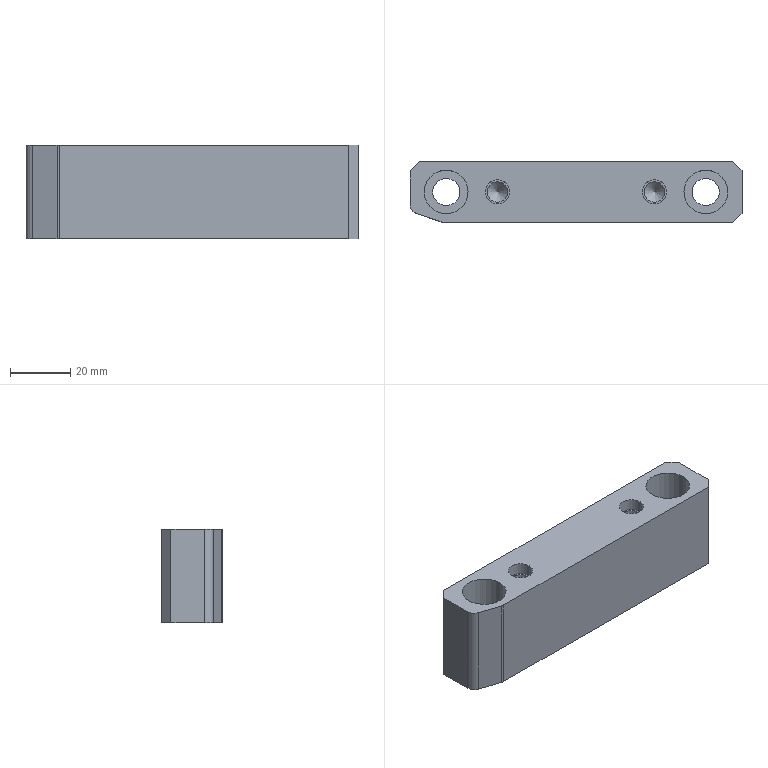Part | NX | features DIE-51 2 | 1 solid | 26 faces | box 110 x 20 x 31 mm | volume 58925 mm3 | plane 14 | cylinder 10 | cone 2 | commonest cylinder face diameters 6 x2 6.806 x2 8 x2 9 x2 14.5 x2
STEP:
#1=CARTESIAN_POINT('',(3332.094,-787.623,884.716));
#2=VERTEX_POINT('',#1);
#3=CARTESIAN_POINT('',(3336.094,-787.623,884.716));
#4=DIRECTION('',(0.,0.,1.));
#5=DIRECTION('',(-1.,0.,0.));
#6=AXIS2_PLACEMENT_3D('',#3,#4,#5);
#7=CIRCLE('',#6,4.);
#8=EDGE_CURVE('',#2,#2,#7,.T.);
#9=ORIENTED_EDGE('',*,*,#8,.F.);
#10=EDGE_LOOP('',(#9));
#11=FACE_BOUND('',#10,.T.);
#12=CARTESIAN_POINT('',(3392.094,-787.623,884.716));
#13=VERTEX_POINT('',#12);
#14=CARTESIAN_POINT('',(3388.094,-787.623,884.716));
#15=DIRECTION('',(0.,0.,-1.));
#16=DIRECTION('',(1.,0.,0.));
#17=AXIS2_PLACEMENT_3D('',#14,#15,#16);
#18=CIRCLE('',#17,4.);
#19=EDGE_CURVE('',#13,#13,#18,.T.);
#20=ORIENTED_EDGE('',*,*,#19,.T.);
#21=EDGE_LOOP('',(#20));
#22=FACE_BOUND('',#21,.T.);
#23=CARTESIAN_POINT('',(3412.344,-787.623,884.716));
#24=VERTEX_POINT('',#23);
#25=CARTESIAN_POINT('',(3405.094,-787.623,884.716));
#26=DIRECTION('',(0.,0.,1.));
#27=DIRECTION('',(1.,0.,0.));
#28=AXIS2_PLACEMENT_3D('',#25,#26,#27);
#29=CIRCLE('',#28,7.25);
#30=EDGE_CURVE('',#24,#24,#29,.T.);
#31=ORIENTED_EDGE('',*,*,#30,.F.);
#32=EDGE_LOOP('',(#31));
#33=FACE_BOUND('',#32,.T.);
#34=CARTESIAN_POINT('',(3326.344,-787.623,884.716));
#35=VERTEX_POINT('',#34);
#36=CARTESIAN_POINT('',(3319.094,-787.623,884.716));
#37=DIRECTION('',(0.,0.,1.));
#38=DIRECTION('',(1.,0.,0.));
#39=AXIS2_PLACEMENT_3D('',#36,#37,#38);
#40=CIRCLE('',#39,7.25);
#41=EDGE_CURVE('',#35,#35,#40,.T.);
#42=ORIENTED_EDGE('',*,*,#41,.F.);
#43=EDGE_LOOP('',(#42));
#44=FACE_BOUND('',#43,.T.);
#45=CARTESIAN_POINT('',(3317.375,-797.469,884.716));
#46=VERTEX_POINT('',#45);
#47=CARTESIAN_POINT('',(3309.145,-794.725,884.716));
#48=VERTEX_POINT('',#47);
#49=CARTESIAN_POINT('',(3313.568,-796.2,884.716));
#50=DIRECTION('',(0.9487,-0.3162,0.));
#51=VECTOR('',#50,1000.);
#52=LINE('',#49,#51);
#53=EDGE_CURVE('',#46,#48,#52,.F.);
#54=ORIENTED_EDGE('',*,*,#53,.F.);
#55=CARTESIAN_POINT('',(3318.324,-797.623,884.716));
#56=VERTEX_POINT('',#55);
#57=CARTESIAN_POINT('',(3318.324,-794.623,884.716));
#58=DIRECTION('',(0.,0.,-1.));
#59=DIRECTION('',(1.,0.,0.));
#60=AXIS2_PLACEMENT_3D('',#57,#58,#59);
#61=CIRCLE('',#60,3.);
#62=EDGE_CURVE('',#56,#46,#61,.T.);
#63=ORIENTED_EDGE('',*,*,#62,.F.);
#64=CARTESIAN_POINT('',(3414.094,-797.623,884.716));
#65=VERTEX_POINT('',#64);
#66=CARTESIAN_POINT('',(3322.094,-797.623,884.716));
#67=DIRECTION('',(1.,0.,0.));
#68=VECTOR('',#67,1000.);
#69=LINE('',#66,#68);
#70=EDGE_CURVE('',#56,#65,#69,.T.);
#71=ORIENTED_EDGE('',*,*,#70,.T.);
#72=CARTESIAN_POINT('',(3417.094,-794.623,884.716));
#73=VERTEX_POINT('',#72);
#74=CARTESIAN_POINT('',(3373.094,-838.623,884.716));
#75=DIRECTION('',(0.7071,0.7071,0.));
#76=VECTOR('',#75,1000.);
#77=LINE('',#74,#76);
#78=EDGE_CURVE('',#73,#65,#77,.F.);
#79=ORIENTED_EDGE('',*,*,#78,.F.);
#80=CARTESIAN_POINT('',(3417.094,-780.623,884.716));
#81=VERTEX_POINT('',#80);
#82=CARTESIAN_POINT('',(3417.094,-787.623,884.716));
#83=DIRECTION('',(0.,1.,0.));
#84=VECTOR('',#83,1000.);
#85=LINE('',#82,#84);
#86=EDGE_CURVE('',#73,#81,#85,.T.);
#87=ORIENTED_EDGE('',*,*,#86,.T.);
#88=CARTESIAN_POINT('',(3414.094,-777.623,884.716));
#89=VERTEX_POINT('',#88);
#90=CARTESIAN_POINT('',(3373.094,-736.623,884.716));
#91=DIRECTION('',(-0.7071,0.7071,0.));
#92=VECTOR('',#91,1000.);
#93=LINE('',#90,#92);
#94=EDGE_CURVE('',#89,#81,#93,.F.);
#95=ORIENTED_EDGE('',*,*,#94,.F.);
#96=CARTESIAN_POINT('',(3310.094,-777.623,884.716));
#97=VERTEX_POINT('',#96);
#98=CARTESIAN_POINT('',(3322.094,-777.623,884.716));
#99=DIRECTION('',(-1.,0.,0.));
#100=VECTOR('',#99,1000.);
#101=LINE('',#98,#100);
#102=EDGE_CURVE('',#89,#97,#101,.T.);
#103=ORIENTED_EDGE('',*,*,#102,.T.);
#104=CARTESIAN_POINT('',(3307.094,-780.623,884.716));
#105=VERTEX_POINT('',#104);
#106=CARTESIAN_POINT('',(3311.094,-776.623,884.716));
#107=DIRECTION('',(-0.7071,-0.7071,0.));
#108=VECTOR('',#107,1000.);
#109=LINE('',#106,#108);
#110=EDGE_CURVE('',#105,#97,#109,.F.);
#111=ORIENTED_EDGE('',*,*,#110,.F.);
#112=CARTESIAN_POINT('',(3307.094,-791.879,884.716));
#113=VERTEX_POINT('',#112);
#114=CARTESIAN_POINT('',(3307.094,-787.623,884.716));
#115=DIRECTION('',(0.,-1.,0.));
#116=VECTOR('',#115,1000.);
#117=LINE('',#114,#116);
#118=EDGE_CURVE('',#105,#113,#117,.T.);
#119=ORIENTED_EDGE('',*,*,#118,.T.);
#120=CARTESIAN_POINT('',(3310.094,-791.879,884.716));
#121=DIRECTION('',(0.,0.,-1.));
#122=DIRECTION('',(1.,0.,0.));
#123=AXIS2_PLACEMENT_3D('',#120,#121,#122);
#124=CIRCLE('',#123,3.);
#125=EDGE_CURVE('',#48,#113,#124,.T.);
#126=ORIENTED_EDGE('',*,*,#125,.F.);
#127=EDGE_LOOP('',(#54,#63,#71,#79,#87,#95,#103,#111,#119,#126));
#128=FACE_BOUND('',#127,.T.);
#129=CARTESIAN_POINT('',(3322.094,-787.623,884.716));
#130=DIRECTION('',(0.,0.,1.));
#131=DIRECTION('',(1.,0.,0.));
#132=AXIS2_PLACEMENT_3D('',#129,#130,#131);
#133=PLANE('',#132);
#134=ADVANCED_FACE('',(#11,#22,#33,#44,#128),#133,.T.);
#135=CARTESIAN_POINT('',(3310.094,-777.623,853.716));
#136=VERTEX_POINT('',#135);
#137=CARTESIAN_POINT('',(3414.094,-777.623,853.716));
#138=VERTEX_POINT('',#137);
#139=CARTESIAN_POINT('',(3322.094,-777.623,853.716));
#140=DIRECTION('',(1.,0.,0.));
#141=VECTOR('',#140,1000.);
#142=LINE('',#139,#141);
#143=EDGE_CURVE('',#136,#138,#142,.T.);
#144=ORIENTED_EDGE('',*,*,#143,.F.);
#145=CARTESIAN_POINT('',(3310.094,-777.623,841.716));
#146=DIRECTION('',(0.,0.,-1.));
#147=VECTOR('',#146,1000.);
#148=LINE('',#145,#147);
#149=EDGE_CURVE('',#97,#136,#148,.T.);
#150=ORIENTED_EDGE('',*,*,#149,.F.);
#151=ORIENTED_EDGE('',*,*,#102,.F.);
#152=CARTESIAN_POINT('',(3414.094,-777.623,841.716));
#153=DIRECTION('',(0.,0.,-1.));
#154=VECTOR('',#153,1000.);
#155=LINE('',#152,#154);
#156=EDGE_CURVE('',#138,#89,#155,.F.);
#157=ORIENTED_EDGE('',*,*,#156,.F.);
#158=EDGE_LOOP('',(#144,#150,#151,#157));
#159=FACE_BOUND('',#158,.T.);
#160=CARTESIAN_POINT('',(3322.094,-777.623,841.716));
#161=DIRECTION('',(0.,1.,0.));
#162=DIRECTION('',(0.,0.,-1.));
#163=AXIS2_PLACEMENT_3D('',#160,#161,#162);
#164=PLANE('',#163);
#165=ADVANCED_FACE('',(#159),#164,.T.);
#166=ORIENTED_EDGE('',*,*,#118,.F.);
#167=CARTESIAN_POINT('',(3307.094,-780.623,853.716));
#168=VERTEX_POINT('',#167);
#169=CARTESIAN_POINT('',(3307.094,-780.623,841.716));
#170=DIRECTION('',(0.,0.,1.));
#171=VECTOR('',#170,1000.);
#172=LINE('',#169,#171);
#173=EDGE_CURVE('',#168,#105,#172,.T.);
#174=ORIENTED_EDGE('',*,*,#173,.F.);
#175=CARTESIAN_POINT('',(3307.094,-791.879,853.716));
#176=VERTEX_POINT('',#175);
#177=CARTESIAN_POINT('',(3307.094,-787.623,853.716));
#178=DIRECTION('',(0.,1.,0.));
#179=VECTOR('',#178,1000.);
#180=LINE('',#177,#179);
#181=EDGE_CURVE('',#176,#168,#180,.T.);
#182=ORIENTED_EDGE('',*,*,#181,.F.);
#183=CARTESIAN_POINT('',(3307.094,-791.879,841.716));
#184=DIRECTION('',(0.,0.,1.));
#185=VECTOR('',#184,1000.);
#186=LINE('',#183,#185);
#187=EDGE_CURVE('',#113,#176,#186,.F.);
#188=ORIENTED_EDGE('',*,*,#187,.F.);
#189=EDGE_LOOP('',(#166,#174,#182,#188));
#190=FACE_BOUND('',#189,.T.);
#191=CARTESIAN_POINT('',(3307.094,-787.623,841.716));
#192=DIRECTION('',(-1.,0.,0.));
#193=DIRECTION('',(0.,0.,1.));
#194=AXIS2_PLACEMENT_3D('',#191,#192,#193);
#195=PLANE('',#194);
#196=ADVANCED_FACE('',(#190),#195,.T.);
#197=CARTESIAN_POINT('',(3414.094,-797.623,853.716));
#198=VERTEX_POINT('',#197);
#199=CARTESIAN_POINT('',(3318.324,-797.623,853.716));
#200=VERTEX_POINT('',#199);
#201=CARTESIAN_POINT('',(3322.094,-797.623,853.716));
#202=DIRECTION('',(-1.,0.,0.));
#203=VECTOR('',#202,1000.);
#204=LINE('',#201,#203);
#205=EDGE_CURVE('',#198,#200,#204,.T.);
#206=ORIENTED_EDGE('',*,*,#205,.F.);
#207=CARTESIAN_POINT('',(3414.094,-797.623,841.716));
#208=DIRECTION('',(0.,0.,1.));
#209=VECTOR('',#208,1000.);
#210=LINE('',#207,#209);
#211=EDGE_CURVE('',#65,#198,#210,.F.);
#212=ORIENTED_EDGE('',*,*,#211,.F.);
#213=ORIENTED_EDGE('',*,*,#70,.F.);
#214=CARTESIAN_POINT('',(3318.324,-797.623,841.716));
#215=DIRECTION('',(0.,0.,-1.));
#216=VECTOR('',#215,1000.);
#217=LINE('',#214,#216);
#218=EDGE_CURVE('',#200,#56,#217,.F.);
#219=ORIENTED_EDGE('',*,*,#218,.F.);
#220=EDGE_LOOP('',(#206,#212,#213,#219));
#221=FACE_BOUND('',#220,.T.);
#222=CARTESIAN_POINT('',(3322.094,-797.623,841.716));
#223=DIRECTION('',(0.,-1.,0.));
#224=DIRECTION('',(0.,0.,1.));
#225=AXIS2_PLACEMENT_3D('',#222,#223,#224);
#226=PLANE('',#225);
#227=ADVANCED_FACE('',(#221),#226,.T.);
#228=CARTESIAN_POINT('',(3400.594,-787.623,853.716));
#229=VERTEX_POINT('',#228);
#230=CARTESIAN_POINT('',(3405.094,-787.623,853.716));
#231=DIRECTION('',(0.,0.,-1.));
#232=DIRECTION('',(-1.,0.,0.));
#233=AXIS2_PLACEMENT_3D('',#230,#231,#232);
#234=CIRCLE('',#233,4.5);
#235=EDGE_CURVE('',#229,#229,#234,.T.);
#236=ORIENTED_EDGE('',*,*,#235,.F.);
#237=EDGE_LOOP('',(#236));
#238=FACE_BOUND('',#237,.T.);
#239=CARTESIAN_POINT('',(3314.594,-787.623,853.716));
#240=VERTEX_POINT('',#239);
#241=CARTESIAN_POINT('',(3319.094,-787.623,853.716));
#242=DIRECTION('',(0.,0.,-1.));
#243=DIRECTION('',(-1.,0.,0.));
#244=AXIS2_PLACEMENT_3D('',#241,#242,#243);
#245=CIRCLE('',#244,4.5);
#246=EDGE_CURVE('',#240,#240,#245,.T.);
#247=ORIENTED_EDGE('',*,*,#246,.F.);
#248=EDGE_LOOP('',(#247));
#249=FACE_BOUND('',#248,.T.);
#250=ORIENTED_EDGE('',*,*,#181,.T.);
#251=CARTESIAN_POINT('',(3307.094,-780.623,853.716));
#252=DIRECTION('',(0.7071,0.7071,0.));
#253=VECTOR('',#252,1000.);
#254=LINE('',#251,#253);
#255=EDGE_CURVE('',#136,#168,#254,.F.);
#256=ORIENTED_EDGE('',*,*,#255,.F.);
#257=ORIENTED_EDGE('',*,*,#143,.T.);
#258=CARTESIAN_POINT('',(3417.094,-780.623,853.716));
#259=VERTEX_POINT('',#258);
#260=CARTESIAN_POINT('',(3414.094,-777.623,853.716));
#261=DIRECTION('',(0.7071,-0.7071,0.));
#262=VECTOR('',#261,1000.);
#263=LINE('',#260,#262);
#264=EDGE_CURVE('',#259,#138,#263,.F.);
#265=ORIENTED_EDGE('',*,*,#264,.F.);
#266=CARTESIAN_POINT('',(3417.094,-794.623,853.716));
#267=VERTEX_POINT('',#266);
#268=CARTESIAN_POINT('',(3417.094,-787.623,853.716));
#269=DIRECTION('',(0.,-1.,0.));
#270=VECTOR('',#269,1000.);
#271=LINE('',#268,#270);
#272=EDGE_CURVE('',#259,#267,#271,.T.);
#273=ORIENTED_EDGE('',*,*,#272,.T.);
#274=CARTESIAN_POINT('',(3417.094,-794.623,853.716));
#275=DIRECTION('',(-0.7071,-0.7071,0.));
#276=VECTOR('',#275,1000.);
#277=LINE('',#274,#276);
#278=EDGE_CURVE('',#198,#267,#277,.F.);
#279=ORIENTED_EDGE('',*,*,#278,.F.);
#280=ORIENTED_EDGE('',*,*,#205,.T.);
#281=CARTESIAN_POINT('',(3317.375,-797.469,853.716));
#282=VERTEX_POINT('',#281);
#283=CARTESIAN_POINT('',(3318.324,-794.623,853.716));
#284=DIRECTION('',(0.,0.,-1.));
#285=DIRECTION('',(-1.,0.,0.));
#286=AXIS2_PLACEMENT_3D('',#283,#284,#285);
#287=CIRCLE('',#286,3.);
#288=EDGE_CURVE('',#282,#200,#287,.F.);
#289=ORIENTED_EDGE('',*,*,#288,.F.);
#290=CARTESIAN_POINT('',(3309.145,-794.725,853.716));
#291=VERTEX_POINT('',#290);
#292=CARTESIAN_POINT('',(3313.568,-796.2,853.716));
#293=DIRECTION('',(-0.9487,0.3162,0.));
#294=VECTOR('',#293,1000.);
#295=LINE('',#292,#294);
#296=EDGE_CURVE('',#291,#282,#295,.F.);
#297=ORIENTED_EDGE('',*,*,#296,.F.);
#298=CARTESIAN_POINT('',(3310.094,-791.879,853.716));
#299=DIRECTION('',(0.,0.,-1.));
#300=DIRECTION('',(-1.,0.,0.));
#301=AXIS2_PLACEMENT_3D('',#298,#299,#300);
#302=CIRCLE('',#301,3.);
#303=EDGE_CURVE('',#176,#291,#302,.F.);
#304=ORIENTED_EDGE('',*,*,#303,.F.);
#305=EDGE_LOOP('',(#250,#256,#257,#265,#273,#279,#280,#289,#297,#304));
#306=FACE_BOUND('',#305,.T.);
#307=CARTESIAN_POINT('',(3322.094,-787.623,853.716));
#308=DIRECTION('',(0.,0.,-1.));
#309=DIRECTION('',(-1.,0.,0.));
#310=AXIS2_PLACEMENT_3D('',#307,#308,#309);
#311=PLANE('',#310);
#312=ADVANCED_FACE('',(#238,#249,#306),#311,.T.);
#313=ORIENTED_EDGE('',*,*,#272,.F.);
#314=CARTESIAN_POINT('',(3417.094,-780.623,841.716));
#315=DIRECTION('',(0.,0.,1.));
#316=VECTOR('',#315,1000.);
#317=LINE('',#314,#316);
#318=EDGE_CURVE('',#81,#259,#317,.F.);
#319=ORIENTED_EDGE('',*,*,#318,.F.);
#320=ORIENTED_EDGE('',*,*,#86,.F.);
#321=CARTESIAN_POINT('',(3417.094,-794.623,841.716));
#322=DIRECTION('',(0.,0.,-1.));
#323=VECTOR('',#322,1000.);
#324=LINE('',#321,#323);
#325=EDGE_CURVE('',#267,#73,#324,.F.);
#326=ORIENTED_EDGE('',*,*,#325,.F.);
#327=EDGE_LOOP('',(#313,#319,#320,#326));
#328=FACE_BOUND('',#327,.T.);
#329=CARTESIAN_POINT('',(3417.094,-787.623,841.716));
#330=DIRECTION('',(1.,0.,0.));
#331=DIRECTION('',(0.,0.,-1.));
#332=AXIS2_PLACEMENT_3D('',#329,#330,#331);
#333=PLANE('',#332);
#334=ADVANCED_FACE('',(#328),#333,.T.);
#335=ORIENTED_EDGE('',*,*,#264,.T.);
#336=ORIENTED_EDGE('',*,*,#156,.T.);
#337=ORIENTED_EDGE('',*,*,#94,.T.);
#338=ORIENTED_EDGE('',*,*,#318,.T.);
#339=EDGE_LOOP('',(#335,#336,#337,#338));
#340=FACE_BOUND('',#339,.T.);
#341=CARTESIAN_POINT('',(3414.094,-777.623,841.716));
#342=DIRECTION('',(-0.7071,-0.7071,0.));
#343=DIRECTION('',(-0.7071,0.7071,0.));
#344=AXIS2_PLACEMENT_3D('',#341,#342,#343);
#345=PLANE('',#344);
#346=ADVANCED_FACE('',(#340),#345,.F.);
#347=ORIENTED_EDGE('',*,*,#255,.T.);
#348=ORIENTED_EDGE('',*,*,#173,.T.);
#349=ORIENTED_EDGE('',*,*,#110,.T.);
#350=ORIENTED_EDGE('',*,*,#149,.T.);
#351=EDGE_LOOP('',(#347,#348,#349,#350));
#352=FACE_BOUND('',#351,.T.);
#353=CARTESIAN_POINT('',(3307.094,-780.623,841.716));
#354=DIRECTION('',(0.7071,-0.7071,0.));
#355=DIRECTION('',(0.,0.,1.));
#356=AXIS2_PLACEMENT_3D('',#353,#354,#355);
#357=PLANE('',#356);
#358=ADVANCED_FACE('',(#352),#357,.F.);
#359=ORIENTED_EDGE('',*,*,#278,.T.);
#360=ORIENTED_EDGE('',*,*,#325,.T.);
#361=ORIENTED_EDGE('',*,*,#78,.T.);
#362=ORIENTED_EDGE('',*,*,#211,.T.);
#363=EDGE_LOOP('',(#359,#360,#361,#362));
#364=FACE_BOUND('',#363,.T.);
#365=CARTESIAN_POINT('',(3417.094,-794.623,841.716));
#366=DIRECTION('',(-0.7071,0.7071,0.));
#367=DIRECTION('',(0.7071,0.7071,0.));
#368=AXIS2_PLACEMENT_3D('',#365,#366,#367);
#369=PLANE('',#368);
#370=ADVANCED_FACE('',(#364),#369,.F.);
#371=ORIENTED_EDGE('',*,*,#296,.T.);
#372=CARTESIAN_POINT('',(3317.375,-797.469,841.716));
#373=DIRECTION('',(0.,0.,1.));
#374=VECTOR('',#373,1000.);
#375=LINE('',#372,#374);
#376=EDGE_CURVE('',#46,#282,#375,.F.);
#377=ORIENTED_EDGE('',*,*,#376,.F.);
#378=ORIENTED_EDGE('',*,*,#53,.T.);
#379=CARTESIAN_POINT('',(3309.145,-794.725,841.716));
#380=DIRECTION('',(0.,0.,-1.));
#381=VECTOR('',#380,1000.);
#382=LINE('',#379,#381);
#383=EDGE_CURVE('',#291,#48,#382,.F.);
#384=ORIENTED_EDGE('',*,*,#383,.F.);
#385=EDGE_LOOP('',(#371,#377,#378,#384));
#386=FACE_BOUND('',#385,.T.);
#387=CARTESIAN_POINT('',(3313.568,-796.2,841.716));
#388=DIRECTION('',(0.3162,0.9487,0.));
#389=DIRECTION('',(0.,0.,1.));
#390=AXIS2_PLACEMENT_3D('',#387,#388,#389);
#391=PLANE('',#390);
#392=ADVANCED_FACE('',(#386),#391,.F.);
#393=ORIENTED_EDGE('',*,*,#125,.T.);
#394=ORIENTED_EDGE('',*,*,#187,.T.);
#395=ORIENTED_EDGE('',*,*,#303,.T.);
#396=ORIENTED_EDGE('',*,*,#383,.T.);
#397=EDGE_LOOP('',(#393,#394,#395,#396));
#398=FACE_BOUND('',#397,.T.);
#399=CARTESIAN_POINT('',(3310.094,-791.879,841.716));
#400=DIRECTION('',(0.,0.,1.));
#401=DIRECTION('',(1.,0.,0.));
#402=AXIS2_PLACEMENT_3D('',#399,#400,#401);
#403=CYLINDRICAL_SURFACE('',#402,3.);
#404=ADVANCED_FACE('',(#398),#403,.T.);
#405=ORIENTED_EDGE('',*,*,#288,.T.);
#406=ORIENTED_EDGE('',*,*,#218,.T.);
#407=ORIENTED_EDGE('',*,*,#62,.T.);
#408=ORIENTED_EDGE('',*,*,#376,.T.);
#409=EDGE_LOOP('',(#405,#406,#407,#408));
#410=FACE_BOUND('',#409,.T.);
#411=CARTESIAN_POINT('',(3318.324,-794.623,841.716));
#412=DIRECTION('',(0.,0.,-1.));
#413=DIRECTION('',(-1.,0.,0.));
#414=AXIS2_PLACEMENT_3D('',#411,#412,#413);
#415=CYLINDRICAL_SURFACE('',#414,3.);
#416=ADVANCED_FACE('',(#410),#415,.T.);
#417=ORIENTED_EDGE('',*,*,#246,.T.);
#418=EDGE_LOOP('',(#417));
#419=FACE_BOUND('',#418,.T.);
#420=CARTESIAN_POINT('',(3323.594,-787.623,871.716));
#421=VERTEX_POINT('',#420);
#422=CARTESIAN_POINT('',(3319.094,-787.623,871.716));
#423=DIRECTION('',(0.,0.,1.));
#424=DIRECTION('',(1.,0.,0.));
#425=AXIS2_PLACEMENT_3D('',#422,#423,#424);
#426=CIRCLE('',#425,4.5);
#427=EDGE_CURVE('',#421,#421,#426,.T.);
#428=ORIENTED_EDGE('',*,*,#427,.T.);
#429=EDGE_LOOP('',(#428));
#430=FACE_BOUND('',#429,.T.);
#431=CARTESIAN_POINT('',(3319.094,-787.623,845.716));
#432=DIRECTION('',(0.,0.,1.));
#433=DIRECTION('',(1.,0.,0.));
#434=AXIS2_PLACEMENT_3D('',#431,#432,#433);
#435=CYLINDRICAL_SURFACE('',#434,4.5);
#436=ADVANCED_FACE('',(#419,#430),#435,.F.);
#437=ORIENTED_EDGE('',*,*,#41,.T.);
#438=EDGE_LOOP('',(#437));
#439=FACE_BOUND('',#438,.T.);
#440=CARTESIAN_POINT('',(3326.344,-787.623,871.716));
#441=VERTEX_POINT('',#440);
#442=CARTESIAN_POINT('',(3319.094,-787.623,871.716));
#443=DIRECTION('',(0.,0.,1.));
#444=DIRECTION('',(1.,0.,0.));
#445=AXIS2_PLACEMENT_3D('',#442,#443,#444);
#446=CIRCLE('',#445,7.25);
#447=EDGE_CURVE('',#441,#441,#446,.F.);
#448=ORIENTED_EDGE('',*,*,#447,.T.);
#449=EDGE_LOOP('',(#448));
#450=FACE_BOUND('',#449,.T.);
#451=CARTESIAN_POINT('',(3319.094,-787.623,871.716));
#452=DIRECTION('',(0.,0.,1.));
#453=DIRECTION('',(1.,0.,0.));
#454=AXIS2_PLACEMENT_3D('',#451,#452,#453);
#455=CYLINDRICAL_SURFACE('',#454,7.25);
#456=ADVANCED_FACE('',(#439,#450),#455,.F.);
#457=ORIENTED_EDGE('',*,*,#427,.F.);
#458=EDGE_LOOP('',(#457));
#459=FACE_BOUND('',#458,.T.);
#460=ORIENTED_EDGE('',*,*,#447,.F.);
#461=EDGE_LOOP('',(#460));
#462=FACE_BOUND('',#461,.T.);
#463=CARTESIAN_POINT('',(3319.094,-787.623,871.716));
#464=DIRECTION('',(0.,0.,1.));
#465=DIRECTION('',(1.,0.,0.));
#466=AXIS2_PLACEMENT_3D('',#463,#464,#465);
#467=PLANE('',#466);
#468=ADVANCED_FACE('',(#459,#462),#467,.T.);
#469=ORIENTED_EDGE('',*,*,#235,.T.);
#470=EDGE_LOOP('',(#469));
#471=FACE_BOUND('',#470,.T.);
#472=CARTESIAN_POINT('',(3409.594,-787.623,871.716));
#473=VERTEX_POINT('',#472);
#474=CARTESIAN_POINT('',(3405.094,-787.623,871.716));
#475=DIRECTION('',(0.,0.,1.));
#476=DIRECTION('',(1.,0.,0.));
#477=AXIS2_PLACEMENT_3D('',#474,#475,#476);
#478=CIRCLE('',#477,4.5);
#479=EDGE_CURVE('',#473,#473,#478,.T.);
#480=ORIENTED_EDGE('',*,*,#479,.T.);
#481=EDGE_LOOP('',(#480));
#482=FACE_BOUND('',#481,.T.);
#483=CARTESIAN_POINT('',(3405.094,-787.623,845.716));
#484=DIRECTION('',(0.,0.,1.));
#485=DIRECTION('',(1.,0.,0.));
#486=AXIS2_PLACEMENT_3D('',#483,#484,#485);
#487=CYLINDRICAL_SURFACE('',#486,4.5);
#488=ADVANCED_FACE('',(#471,#482),#487,.F.);
#489=ORIENTED_EDGE('',*,*,#30,.T.);
#490=EDGE_LOOP('',(#489));
#491=FACE_BOUND('',#490,.T.);
#492=CARTESIAN_POINT('',(3412.344,-787.623,871.716));
#493=VERTEX_POINT('',#492);
#494=CARTESIAN_POINT('',(3405.094,-787.623,871.716));
#495=DIRECTION('',(0.,0.,1.));
#496=DIRECTION('',(1.,0.,0.));
#497=AXIS2_PLACEMENT_3D('',#494,#495,#496);
#498=CIRCLE('',#497,7.25);
#499=EDGE_CURVE('',#493,#493,#498,.F.);
#500=ORIENTED_EDGE('',*,*,#499,.T.);
#501=EDGE_LOOP('',(#500));
#502=FACE_BOUND('',#501,.T.);
#503=CARTESIAN_POINT('',(3405.094,-787.623,871.716));
#504=DIRECTION('',(0.,0.,1.));
#505=DIRECTION('',(1.,0.,0.));
#506=AXIS2_PLACEMENT_3D('',#503,#504,#505);
#507=CYLINDRICAL_SURFACE('',#506,7.25);
#508=ADVANCED_FACE('',(#491,#502),#507,.F.);
#509=ORIENTED_EDGE('',*,*,#479,.F.);
#510=EDGE_LOOP('',(#509));
#511=FACE_BOUND('',#510,.T.);
#512=ORIENTED_EDGE('',*,*,#499,.F.);
#513=EDGE_LOOP('',(#512));
#514=FACE_BOUND('',#513,.T.);
#515=CARTESIAN_POINT('',(3405.094,-787.623,871.716));
#516=DIRECTION('',(0.,0.,1.));
#517=DIRECTION('',(1.,0.,0.));
#518=AXIS2_PLACEMENT_3D('',#515,#516,#517);
#519=PLANE('',#518);
#520=ADVANCED_FACE('',(#511,#514),#519,.T.);
#521=CARTESIAN_POINT('',(3384.691,-787.623,880.716));
#522=VERTEX_POINT('',#521);
#523=CARTESIAN_POINT('',(3388.094,-787.623,880.716));
#524=DIRECTION('',(0.,0.,-1.));
#525=DIRECTION('',(-1.,0.,0.));
#526=AXIS2_PLACEMENT_3D('',#523,#524,#525);
#527=CIRCLE('',#526,3.403);
#528=EDGE_CURVE('',#522,#522,#527,.T.);
#529=ORIENTED_EDGE('',*,*,#528,.F.);
#530=EDGE_LOOP('',(#529));
#531=FACE_BOUND('',#530,.T.);
#532=CARTESIAN_POINT('',(3384.691,-787.623,864.716));
#533=VERTEX_POINT('',#532);
#534=CARTESIAN_POINT('',(3388.094,-787.623,864.716));
#535=DIRECTION('',(0.,0.,-1.));
#536=DIRECTION('',(-1.,0.,0.));
#537=AXIS2_PLACEMENT_3D('',#534,#535,#536);
#538=CIRCLE('',#537,3.403);
#539=EDGE_CURVE('',#533,#533,#538,.T.);
#540=ORIENTED_EDGE('',*,*,#539,.T.);
#541=EDGE_LOOP('',(#540));
#542=FACE_BOUND('',#541,.T.);
#543=CARTESIAN_POINT('',(3388.094,-787.623,889.716));
#544=DIRECTION('',(0.,0.,-1.));
#545=DIRECTION('',(1.,0.,0.));
#546=AXIS2_PLACEMENT_3D('',#543,#544,#545);
#547=CYLINDRICAL_SURFACE('',#546,3.403);
#548=ADVANCED_FACE('',(#531,#542),#547,.F.);
#549=CARTESIAN_POINT('',(3388.094,-787.623,861.313));
#550=VERTEX_POINT('',#549);
#551=VERTEX_LOOP('',#550);
#552=FACE_BOUND('',#551,.T.);
#553=ORIENTED_EDGE('',*,*,#539,.F.);
#554=EDGE_LOOP('',(#553));
#555=FACE_BOUND('',#554,.T.);
#556=CARTESIAN_POINT('',(3388.094,-787.623,864.716));
#557=DIRECTION('',(0.,0.,1.));
#558=DIRECTION('',(1.,0.,0.));
#559=AXIS2_PLACEMENT_3D('',#556,#557,#558);
#560=CONICAL_SURFACE('',#559,3.403,0.7854);
#561=ADVANCED_FACE('',(#552,#555),#560,.F.);
#562=ORIENTED_EDGE('',*,*,#528,.T.);
#563=EDGE_LOOP('',(#562));
#564=FACE_BOUND('',#563,.T.);
#565=CARTESIAN_POINT('',(3392.094,-787.623,880.716));
#566=VERTEX_POINT('',#565);
#567=CARTESIAN_POINT('',(3388.094,-787.623,880.716));
#568=DIRECTION('',(0.,0.,1.));
#569=DIRECTION('',(1.,0.,0.));
#570=AXIS2_PLACEMENT_3D('',#567,#568,#569);
#571=CIRCLE('',#570,4.);
#572=EDGE_CURVE('',#566,#566,#571,.F.);
#573=ORIENTED_EDGE('',*,*,#572,.F.);
#574=EDGE_LOOP('',(#573));
#575=FACE_BOUND('',#574,.T.);
#576=CARTESIAN_POINT('',(3388.094,-787.623,880.716));
#577=DIRECTION('',(0.,0.,-1.));
#578=DIRECTION('',(-1.,0.,0.));
#579=AXIS2_PLACEMENT_3D('',#576,#577,#578);
#580=PLANE('',#579);
#581=ADVANCED_FACE('',(#564,#575),#580,.F.);
#582=ORIENTED_EDGE('',*,*,#572,.T.);
#583=EDGE_LOOP('',(#582));
#584=FACE_BOUND('',#583,.T.);
#585=ORIENTED_EDGE('',*,*,#19,.F.);
#586=EDGE_LOOP('',(#585));
#587=FACE_BOUND('',#586,.T.);
#588=CARTESIAN_POINT('',(3388.094,-787.623,884.716));
#589=DIRECTION('',(0.,0.,-1.));
#590=DIRECTION('',(1.,0.,0.));
#591=AXIS2_PLACEMENT_3D('',#588,#589,#590);
#592=CYLINDRICAL_SURFACE('',#591,4.);
#593=ADVANCED_FACE('',(#584,#587),#592,.F.);
#594=CARTESIAN_POINT('',(3339.497,-787.623,880.716));
#595=VERTEX_POINT('',#594);
#596=CARTESIAN_POINT('',(3336.094,-787.623,880.716));
#597=DIRECTION('',(0.,0.,1.));
#598=DIRECTION('',(1.,0.,0.));
#599=AXIS2_PLACEMENT_3D('',#596,#597,#598);
#600=CIRCLE('',#599,3.403);
#601=EDGE_CURVE('',#595,#595,#600,.T.);
#602=ORIENTED_EDGE('',*,*,#601,.T.);
#603=EDGE_LOOP('',(#602));
#604=FACE_BOUND('',#603,.T.);
#605=CARTESIAN_POINT('',(3339.497,-787.623,864.716));
#606=VERTEX_POINT('',#605);
#607=CARTESIAN_POINT('',(3336.094,-787.623,864.716));
#608=DIRECTION('',(0.,0.,1.));
#609=DIRECTION('',(1.,0.,0.));
#610=AXIS2_PLACEMENT_3D('',#607,#608,#609);
#611=CIRCLE('',#610,3.403);
#612=EDGE_CURVE('',#606,#606,#611,.T.);
#613=ORIENTED_EDGE('',*,*,#612,.F.);
#614=EDGE_LOOP('',(#613));
#615=FACE_BOUND('',#614,.T.);
#616=CARTESIAN_POINT('',(3336.094,-787.623,889.716));
#617=DIRECTION('',(0.,0.,-1.));
#618=DIRECTION('',(-1.,0.,0.));
#619=AXIS2_PLACEMENT_3D('',#616,#617,#618);
#620=CYLINDRICAL_SURFACE('',#619,3.403);
#621=ADVANCED_FACE('',(#604,#615),#620,.F.);
#622=CARTESIAN_POINT('',(3336.094,-787.623,861.313));
#623=VERTEX_POINT('',#622);
#624=VERTEX_LOOP('',#623);
#625=FACE_BOUND('',#624,.T.);
#626=ORIENTED_EDGE('',*,*,#612,.T.);
#627=EDGE_LOOP('',(#626));
#628=FACE_BOUND('',#627,.T.);
#629=CARTESIAN_POINT('',(3336.094,-787.623,864.716));
#630=DIRECTION('',(0.,0.,1.));
#631=DIRECTION('',(-1.,0.,0.));
#632=AXIS2_PLACEMENT_3D('',#629,#630,#631);
#633=CONICAL_SURFACE('',#632,3.403,0.7854);
#634=ADVANCED_FACE('',(#625,#628),#633,.F.);
#635=ORIENTED_EDGE('',*,*,#601,.F.);
#636=EDGE_LOOP('',(#635));
#637=FACE_BOUND('',#636,.T.);
#638=CARTESIAN_POINT('',(3332.094,-787.623,880.716));
#639=VERTEX_POINT('',#638);
#640=CARTESIAN_POINT('',(3336.094,-787.623,880.716));
#641=DIRECTION('',(0.,0.,-1.));
#642=DIRECTION('',(-1.,0.,0.));
#643=AXIS2_PLACEMENT_3D('',#640,#641,#642);
#644=CIRCLE('',#643,4.);
#645=EDGE_CURVE('',#639,#639,#644,.F.);
#646=ORIENTED_EDGE('',*,*,#645,.T.);
#647=EDGE_LOOP('',(#646));
#648=FACE_BOUND('',#647,.T.);
#649=CARTESIAN_POINT('',(3336.094,-787.623,880.716));
#650=DIRECTION('',(0.,0.,-1.));
#651=DIRECTION('',(1.,0.,0.));
#652=AXIS2_PLACEMENT_3D('',#649,#650,#651);
#653=PLANE('',#652);
#654=ADVANCED_FACE('',(#637,#648),#653,.F.);
#655=ORIENTED_EDGE('',*,*,#645,.F.);
#656=EDGE_LOOP('',(#655));
#657=FACE_BOUND('',#656,.T.);
#658=ORIENTED_EDGE('',*,*,#8,.T.);
#659=EDGE_LOOP('',(#658));
#660=FACE_BOUND('',#659,.T.);
#661=CARTESIAN_POINT('',(3336.094,-787.623,884.716));
#662=DIRECTION('',(0.,0.,-1.));
#663=DIRECTION('',(-1.,0.,0.));
#664=AXIS2_PLACEMENT_3D('',#661,#662,#663);
#665=CYLINDRICAL_SURFACE('',#664,4.);
#666=ADVANCED_FACE('',(#657,#660),#665,.F.);
#667=CLOSED_SHELL('',(#134,#165,#196,#227,#312,#334,#346,#358,#370,#392,#404,#416,#436,#456,#468,#488,#508,#520,#548,#561,#581,#593,#621,#634,#654,#666));
#668=MANIFOLD_SOLID_BREP('',#667);
#669=(LENGTH_UNIT()NAMED_UNIT(*)SI_UNIT(.MILLI.,.METRE.));
#670=UNCERTAINTY_MEASURE_WITH_UNIT(LENGTH_MEASURE(0.00001),#669,'','');
#671=(NAMED_UNIT(*)PLANE_ANGLE_UNIT()SI_UNIT($,.RADIAN.));
#672=(NAMED_UNIT(*)SI_UNIT($,.STERADIAN.)SOLID_ANGLE_UNIT());
#673=(GEOMETRIC_REPRESENTATION_CONTEXT(3)GLOBAL_UNCERTAINTY_ASSIGNED_CONTEXT((#670))GLOBAL_UNIT_ASSIGNED_CONTEXT((#669,#671,#672))REPRESENTATION_CONTEXT('',''));
#674=ADVANCED_BREP_SHAPE_REPRESENTATION('',(#668),#673);